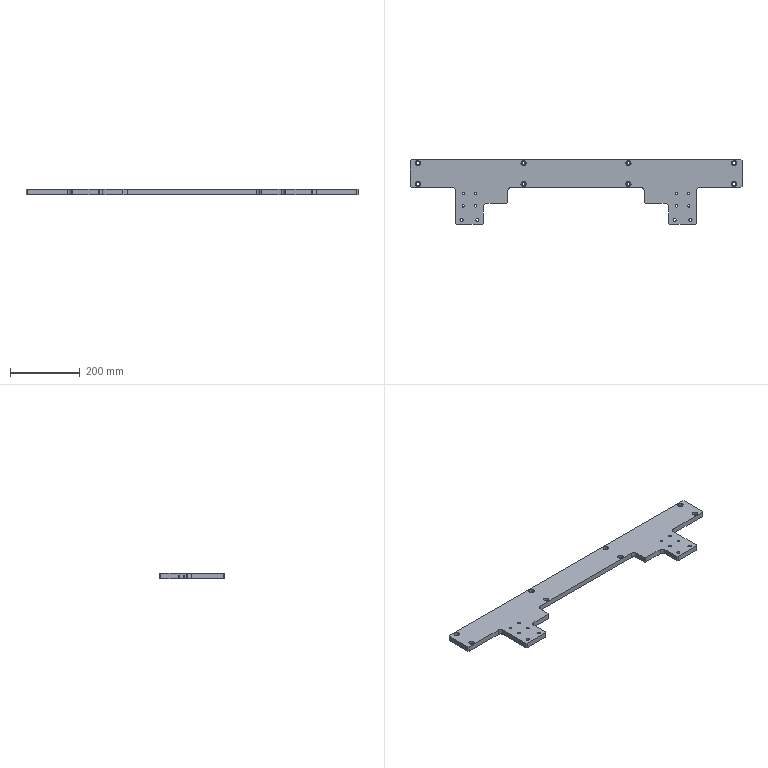Part | SolidWorks | features HoleWzd 5, MirrorPattern 3, Chamfer 2, Fillet 2, ICE 2, Extrusion 1 | 1 solid | 114 faces | box 950 x 185 x 15 mm | volume 1463196 mm3 | cylinder 70 | plane 36 | cone 8 | commonest cylinder face diameters 9 x24 7 x16 15 x16 4.2 x8 20 x6